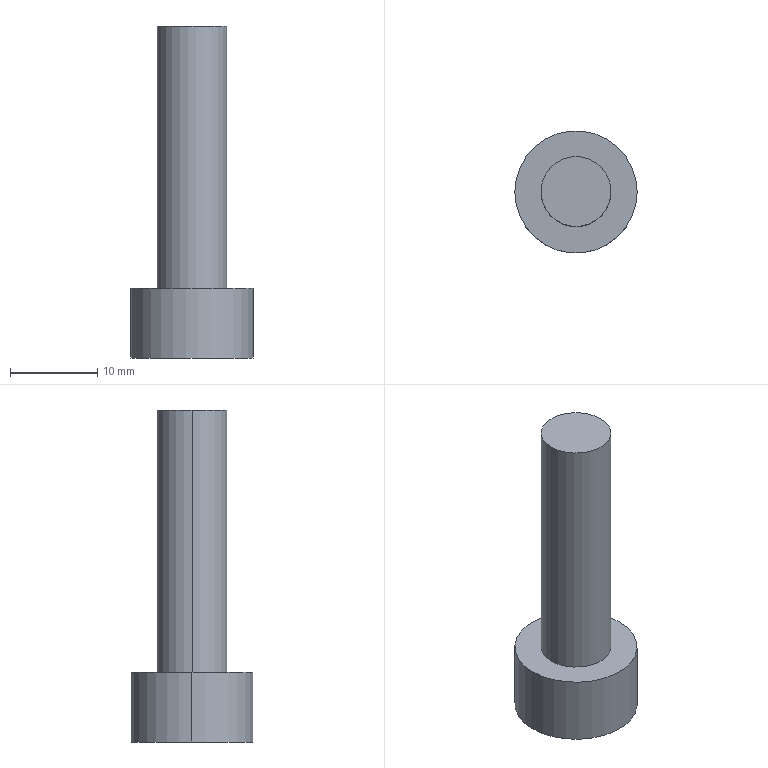Part | STEP file | LG M8_3F | 1 solid | 14 faces | box 14 x 14 x 38 mm | volume 2614 mm3 | plane 10 | cylinder 4 | commonest cylinder face diameters 8 x2 14 x2
STEP:
#1=CARTESIAN_POINT('',(0.,0.,0.));
#2=DIRECTION('',(0.,0.,1.));
#3=DIRECTION('',(1.,0.,0.));
#4=AXIS2_PLACEMENT_3D('',#1,#2,#3);
#5=CARTESIAN_POINT('',(4.,0.,30.));
#6=VERTEX_POINT('',#5);
#7=CARTESIAN_POINT('',(-4.,0.,30.));
#8=VERTEX_POINT('',#7);
#9=CARTESIAN_POINT('',(0.,0.,30.));
#10=DIRECTION('',(0.,0.,1.));
#11=DIRECTION('',(1.,0.,0.));
#12=AXIS2_PLACEMENT_3D('',#9,#10,#11);
#13=CIRCLE('',#12,4.);
#14=CARTESIAN_POINT('',(0.,0.,30.));
#15=DIRECTION('',(0.,0.,-1.));
#16=DIRECTION('',(-1.,0.,0.));
#17=AXIS2_PLACEMENT_3D('',#14,#15,#16);
#18=CYLINDRICAL_SURFACE('',#17,4.);
#19=CARTESIAN_POINT('',(3.142,0.));
#20=DIRECTION('',(-1.,0.));
#21=VECTOR('',#20,1.);
#22=LINE('',#19,#21);
#23=(GEOMETRIC_REPRESENTATION_CONTEXT(2)PARAMETRIC_REPRESENTATION_CONTEXT()REPRESENTATION_CONTEXT('',''));
#24=DEFINITIONAL_REPRESENTATION('',(#22),#23);
#25=PCURVE('',#18,#24);
#26=CARTESIAN_POINT('',(0.,0.,30.));
#27=DIRECTION('',(0.,0.,1.));
#28=DIRECTION('',(1.,0.,0.));
#29=AXIS2_PLACEMENT_3D('',#26,#27,#28);
#30=PLANE('',#29);
#31=CARTESIAN_POINT('',(0.,0.));
#32=DIRECTION('',(1.,0.));
#33=AXIS2_PLACEMENT_2D('',#31,#32);
#34=CIRCLE('',#33,4.);
#35=(GEOMETRIC_REPRESENTATION_CONTEXT(2)PARAMETRIC_REPRESENTATION_CONTEXT()REPRESENTATION_CONTEXT('',''));
#36=DEFINITIONAL_REPRESENTATION('',(#34),#35);
#37=PCURVE('',#30,#36);
#38=SURFACE_CURVE('',#13,(#25,#37),.PCURVE_S1.);
#39=EDGE_CURVE('',#6,#8,#38,.T.);
#40=ORIENTED_EDGE('',*,*,#39,.F.);
#41=CARTESIAN_POINT('',(4.,0.,0.));
#42=VERTEX_POINT('',#41);
#43=CARTESIAN_POINT('',(4.,0.,30.));
#44=DIRECTION('',(0.,0.,-1.));
#45=VECTOR('',#44,1.);
#46=LINE('',#43,#45);
#47=CARTESIAN_POINT('',(3.142,0.));
#48=DIRECTION('',(0.,1.));
#49=VECTOR('',#48,1.);
#50=LINE('',#47,#49);
#51=(GEOMETRIC_REPRESENTATION_CONTEXT(2)PARAMETRIC_REPRESENTATION_CONTEXT()REPRESENTATION_CONTEXT('',''));
#52=DEFINITIONAL_REPRESENTATION('',(#50),#51);
#53=PCURVE('',#18,#52);
#54=CARTESIAN_POINT('',(0.,0.,30.));
#55=DIRECTION('',(0.,0.,-1.));
#56=DIRECTION('',(-1.,0.,0.));
#57=AXIS2_PLACEMENT_3D('',#54,#55,#56);
#58=CYLINDRICAL_SURFACE('',#57,4.);
#59=CARTESIAN_POINT('',(3.142,0.));
#60=DIRECTION('',(0.,1.));
#61=VECTOR('',#60,1.);
#62=LINE('',#59,#61);
#63=(GEOMETRIC_REPRESENTATION_CONTEXT(2)PARAMETRIC_REPRESENTATION_CONTEXT()REPRESENTATION_CONTEXT('',''));
#64=DEFINITIONAL_REPRESENTATION('',(#62),#63);
#65=PCURVE('',#58,#64);
#66=SURFACE_CURVE('',#46,(#53,#65),.PCURVE_S1.);
#67=EDGE_CURVE('',#6,#42,#66,.T.);
#68=ORIENTED_EDGE('',*,*,#67,.T.);
#69=CARTESIAN_POINT('',(-4.,0.,0.));
#70=VERTEX_POINT('',#69);
#71=CARTESIAN_POINT('',(0.,0.,0.));
#72=DIRECTION('',(0.,0.,1.));
#73=DIRECTION('',(1.,0.,0.));
#74=AXIS2_PLACEMENT_3D('',#71,#72,#73);
#75=CIRCLE('',#74,4.);
#76=CARTESIAN_POINT('',(3.142,30.));
#77=DIRECTION('',(-1.,0.));
#78=VECTOR('',#77,1.);
#79=LINE('',#76,#78);
#80=(GEOMETRIC_REPRESENTATION_CONTEXT(2)PARAMETRIC_REPRESENTATION_CONTEXT()REPRESENTATION_CONTEXT('',''));
#81=DEFINITIONAL_REPRESENTATION('',(#79),#80);
#82=PCURVE('',#18,#81);
#83=CARTESIAN_POINT('',(0.,0.,0.));
#84=DIRECTION('',(0.,0.,1.));
#85=DIRECTION('',(1.,0.,0.));
#86=AXIS2_PLACEMENT_3D('',#83,#84,#85);
#87=PLANE('',#86);
#88=CARTESIAN_POINT('',(0.,0.));
#89=DIRECTION('',(1.,0.));
#90=AXIS2_PLACEMENT_2D('',#88,#89);
#91=CIRCLE('',#90,4.);
#92=(GEOMETRIC_REPRESENTATION_CONTEXT(2)PARAMETRIC_REPRESENTATION_CONTEXT()REPRESENTATION_CONTEXT('',''));
#93=DEFINITIONAL_REPRESENTATION('',(#91),#92);
#94=PCURVE('',#87,#93);
#95=SURFACE_CURVE('',#75,(#82,#94),.PCURVE_S1.);
#96=EDGE_CURVE('',#42,#70,#95,.T.);
#97=ORIENTED_EDGE('',*,*,#96,.T.);
#98=CARTESIAN_POINT('',(-4.,0.,30.));
#99=DIRECTION('',(0.,0.,-1.));
#100=VECTOR('',#99,1.);
#101=LINE('',#98,#100);
#102=CARTESIAN_POINT('',(0.,0.));
#103=DIRECTION('',(0.,1.));
#104=VECTOR('',#103,1.);
#105=LINE('',#102,#104);
#106=(GEOMETRIC_REPRESENTATION_CONTEXT(2)PARAMETRIC_REPRESENTATION_CONTEXT()REPRESENTATION_CONTEXT('',''));
#107=DEFINITIONAL_REPRESENTATION('',(#105),#106);
#108=PCURVE('',#18,#107);
#109=CARTESIAN_POINT('',(6.283,0.));
#110=DIRECTION('',(0.,1.));
#111=VECTOR('',#110,1.);
#112=LINE('',#109,#111);
#113=(GEOMETRIC_REPRESENTATION_CONTEXT(2)PARAMETRIC_REPRESENTATION_CONTEXT()REPRESENTATION_CONTEXT('',''));
#114=DEFINITIONAL_REPRESENTATION('',(#112),#113);
#115=PCURVE('',#58,#114);
#116=SURFACE_CURVE('',#101,(#108,#115),.PCURVE_S1.);
#117=EDGE_CURVE('',#8,#70,#116,.T.);
#118=ORIENTED_EDGE('',*,*,#117,.F.);
#119=EDGE_LOOP('',(#40,#68,#97,#118));
#120=FACE_BOUND('',#119,.T.);
#121=ADVANCED_FACE('',(#120),#18,.T.);
#122=CARTESIAN_POINT('',(7.,0.,-8.));
#123=VERTEX_POINT('',#122);
#124=CARTESIAN_POINT('',(-7.,0.,-8.));
#125=VERTEX_POINT('',#124);
#126=CARTESIAN_POINT('',(0.,0.,-8.));
#127=DIRECTION('',(0.,0.,1.));
#128=DIRECTION('',(1.,0.,0.));
#129=AXIS2_PLACEMENT_3D('',#126,#127,#128);
#130=CIRCLE('',#129,7.);
#131=CARTESIAN_POINT('',(0.,0.,-8.));
#132=DIRECTION('',(0.,0.,1.));
#133=DIRECTION('',(1.,0.,0.));
#134=AXIS2_PLACEMENT_3D('',#131,#132,#133);
#135=CYLINDRICAL_SURFACE('',#134,7.);
#136=CARTESIAN_POINT('',(0.,0.));
#137=DIRECTION('',(1.,0.));
#138=VECTOR('',#137,1.);
#139=LINE('',#136,#138);
#140=(GEOMETRIC_REPRESENTATION_CONTEXT(2)PARAMETRIC_REPRESENTATION_CONTEXT()REPRESENTATION_CONTEXT('',''));
#141=DEFINITIONAL_REPRESENTATION('',(#139),#140);
#142=PCURVE('',#135,#141);
#143=CARTESIAN_POINT('',(0.,0.,-8.));
#144=DIRECTION('',(0.,0.,1.));
#145=DIRECTION('',(1.,0.,0.));
#146=AXIS2_PLACEMENT_3D('',#143,#144,#145);
#147=PLANE('',#146);
#148=CARTESIAN_POINT('',(0.,0.));
#149=DIRECTION('',(1.,0.));
#150=AXIS2_PLACEMENT_2D('',#148,#149);
#151=CIRCLE('',#150,7.);
#152=(GEOMETRIC_REPRESENTATION_CONTEXT(2)PARAMETRIC_REPRESENTATION_CONTEXT()REPRESENTATION_CONTEXT('',''));
#153=DEFINITIONAL_REPRESENTATION('',(#151),#152);
#154=PCURVE('',#147,#153);
#155=SURFACE_CURVE('',#130,(#142,#154),.PCURVE_S1.);
#156=EDGE_CURVE('',#123,#125,#155,.T.);
#157=ORIENTED_EDGE('',*,*,#156,.T.);
#158=CARTESIAN_POINT('',(-7.,0.,0.));
#159=VERTEX_POINT('',#158);
#160=CARTESIAN_POINT('',(-7.,0.,-8.));
#161=DIRECTION('',(0.,0.,1.));
#162=VECTOR('',#161,1.);
#163=LINE('',#160,#162);
#164=CARTESIAN_POINT('',(3.142,0.));
#165=DIRECTION('',(0.,1.));
#166=VECTOR('',#165,1.);
#167=LINE('',#164,#166);
#168=(GEOMETRIC_REPRESENTATION_CONTEXT(2)PARAMETRIC_REPRESENTATION_CONTEXT()REPRESENTATION_CONTEXT('',''));
#169=DEFINITIONAL_REPRESENTATION('',(#167),#168);
#170=PCURVE('',#135,#169);
#171=CARTESIAN_POINT('',(0.,0.,-8.));
#172=DIRECTION('',(0.,0.,1.));
#173=DIRECTION('',(1.,0.,0.));
#174=AXIS2_PLACEMENT_3D('',#171,#172,#173);
#175=CYLINDRICAL_SURFACE('',#174,7.);
#176=CARTESIAN_POINT('',(3.142,0.));
#177=DIRECTION('',(0.,1.));
#178=VECTOR('',#177,1.);
#179=LINE('',#176,#178);
#180=(GEOMETRIC_REPRESENTATION_CONTEXT(2)PARAMETRIC_REPRESENTATION_CONTEXT()REPRESENTATION_CONTEXT('',''));
#181=DEFINITIONAL_REPRESENTATION('',(#179),#180);
#182=PCURVE('',#175,#181);
#183=SURFACE_CURVE('',#163,(#170,#182),.PCURVE_S1.);
#184=EDGE_CURVE('',#125,#159,#183,.T.);
#185=ORIENTED_EDGE('',*,*,#184,.T.);
#186=CARTESIAN_POINT('',(7.,0.,0.));
#187=VERTEX_POINT('',#186);
#188=CARTESIAN_POINT('',(0.,0.,0.));
#189=DIRECTION('',(0.,0.,1.));
#190=DIRECTION('',(1.,0.,0.));
#191=AXIS2_PLACEMENT_3D('',#188,#189,#190);
#192=CIRCLE('',#191,7.);
#193=CARTESIAN_POINT('',(0.,8.));
#194=DIRECTION('',(1.,0.));
#195=VECTOR('',#194,1.);
#196=LINE('',#193,#195);
#197=(GEOMETRIC_REPRESENTATION_CONTEXT(2)PARAMETRIC_REPRESENTATION_CONTEXT()REPRESENTATION_CONTEXT('',''));
#198=DEFINITIONAL_REPRESENTATION('',(#196),#197);
#199=PCURVE('',#135,#198);
#200=CARTESIAN_POINT('',(0.,0.));
#201=DIRECTION('',(1.,0.));
#202=AXIS2_PLACEMENT_2D('',#200,#201);
#203=CIRCLE('',#202,7.);
#204=(GEOMETRIC_REPRESENTATION_CONTEXT(2)PARAMETRIC_REPRESENTATION_CONTEXT()REPRESENTATION_CONTEXT('',''));
#205=DEFINITIONAL_REPRESENTATION('',(#203),#204);
#206=PCURVE('',#87,#205);
#207=SURFACE_CURVE('',#192,(#199,#206),.PCURVE_S1.);
#208=EDGE_CURVE('',#187,#159,#207,.T.);
#209=ORIENTED_EDGE('',*,*,#208,.F.);
#210=CARTESIAN_POINT('',(7.,0.,-8.));
#211=DIRECTION('',(0.,0.,1.));
#212=VECTOR('',#211,1.);
#213=LINE('',#210,#212);
#214=CARTESIAN_POINT('',(0.,0.));
#215=DIRECTION('',(0.,1.));
#216=VECTOR('',#215,1.);
#217=LINE('',#214,#216);
#218=(GEOMETRIC_REPRESENTATION_CONTEXT(2)PARAMETRIC_REPRESENTATION_CONTEXT()REPRESENTATION_CONTEXT('',''));
#219=DEFINITIONAL_REPRESENTATION('',(#217),#218);
#220=PCURVE('',#135,#219);
#221=CARTESIAN_POINT('',(6.283,0.));
#222=DIRECTION('',(0.,1.));
#223=VECTOR('',#222,1.);
#224=LINE('',#221,#223);
#225=(GEOMETRIC_REPRESENTATION_CONTEXT(2)PARAMETRIC_REPRESENTATION_CONTEXT()REPRESENTATION_CONTEXT('',''));
#226=DEFINITIONAL_REPRESENTATION('',(#224),#225);
#227=PCURVE('',#175,#226);
#228=SURFACE_CURVE('',#213,(#220,#227),.PCURVE_S1.);
#229=EDGE_CURVE('',#123,#187,#228,.T.);
#230=ORIENTED_EDGE('',*,*,#229,.F.);
#231=EDGE_LOOP('',(#157,#185,#209,#230));
#232=FACE_BOUND('',#231,.T.);
#233=ADVANCED_FACE('',(#232),#135,.T.);
#234=ORIENTED_EDGE('',*,*,#208,.T.);
#235=CARTESIAN_POINT('',(0.,0.,0.));
#236=DIRECTION('',(0.,0.,1.));
#237=DIRECTION('',(1.,0.,0.));
#238=AXIS2_PLACEMENT_3D('',#235,#236,#237);
#239=CIRCLE('',#238,7.);
#240=CARTESIAN_POINT('',(0.,0.));
#241=DIRECTION('',(1.,0.));
#242=AXIS2_PLACEMENT_2D('',#240,#241);
#243=CIRCLE('',#242,7.);
#244=(GEOMETRIC_REPRESENTATION_CONTEXT(2)PARAMETRIC_REPRESENTATION_CONTEXT()REPRESENTATION_CONTEXT('',''));
#245=DEFINITIONAL_REPRESENTATION('',(#243),#244);
#246=PCURVE('',#87,#245);
#247=CARTESIAN_POINT('',(0.,8.));
#248=DIRECTION('',(1.,0.));
#249=VECTOR('',#248,1.);
#250=LINE('',#247,#249);
#251=(GEOMETRIC_REPRESENTATION_CONTEXT(2)PARAMETRIC_REPRESENTATION_CONTEXT()REPRESENTATION_CONTEXT('',''));
#252=DEFINITIONAL_REPRESENTATION('',(#250),#251);
#253=PCURVE('',#175,#252);
#254=SURFACE_CURVE('',#239,(#246,#253),.PCURVE_S1.);
#255=EDGE_CURVE('',#159,#187,#254,.T.);
#256=ORIENTED_EDGE('',*,*,#255,.T.);
#257=EDGE_LOOP('',(#234,#256));
#258=FACE_BOUND('',#257,.T.);
#259=CARTESIAN_POINT('',(0.,0.,0.));
#260=DIRECTION('',(0.,0.,1.));
#261=DIRECTION('',(1.,0.,0.));
#262=AXIS2_PLACEMENT_3D('',#259,#260,#261);
#263=CIRCLE('',#262,4.);
#264=CARTESIAN_POINT('',(0.,0.));
#265=DIRECTION('',(1.,0.));
#266=AXIS2_PLACEMENT_2D('',#264,#265);
#267=CIRCLE('',#266,4.);
#268=(GEOMETRIC_REPRESENTATION_CONTEXT(2)PARAMETRIC_REPRESENTATION_CONTEXT()REPRESENTATION_CONTEXT('',''));
#269=DEFINITIONAL_REPRESENTATION('',(#267),#268);
#270=PCURVE('',#87,#269);
#271=CARTESIAN_POINT('',(9.425,30.));
#272=DIRECTION('',(-1.,0.));
#273=VECTOR('',#272,1.);
#274=LINE('',#271,#273);
#275=(GEOMETRIC_REPRESENTATION_CONTEXT(2)PARAMETRIC_REPRESENTATION_CONTEXT()REPRESENTATION_CONTEXT('',''));
#276=DEFINITIONAL_REPRESENTATION('',(#274),#275);
#277=PCURVE('',#58,#276);
#278=SURFACE_CURVE('',#263,(#270,#277),.PCURVE_S1.);
#279=EDGE_CURVE('',#70,#42,#278,.T.);
#280=ORIENTED_EDGE('',*,*,#279,.F.);
#281=ORIENTED_EDGE('',*,*,#96,.F.);
#282=EDGE_LOOP('',(#280,#281));
#283=FACE_BOUND('',#282,.T.);
#284=ADVANCED_FACE('',(#258,#283),#87,.T.);
#285=ORIENTED_EDGE('',*,*,#184,.F.);
#286=CARTESIAN_POINT('',(0.,0.,-8.));
#287=DIRECTION('',(0.,0.,1.));
#288=DIRECTION('',(1.,0.,0.));
#289=AXIS2_PLACEMENT_3D('',#286,#287,#288);
#290=CIRCLE('',#289,7.);
#291=CARTESIAN_POINT('',(0.,0.));
#292=DIRECTION('',(1.,0.));
#293=VECTOR('',#292,1.);
#294=LINE('',#291,#293);
#295=(GEOMETRIC_REPRESENTATION_CONTEXT(2)PARAMETRIC_REPRESENTATION_CONTEXT()REPRESENTATION_CONTEXT('',''));
#296=DEFINITIONAL_REPRESENTATION('',(#294),#295);
#297=PCURVE('',#175,#296);
#298=CARTESIAN_POINT('',(0.,0.));
#299=DIRECTION('',(1.,0.));
#300=AXIS2_PLACEMENT_2D('',#298,#299);
#301=CIRCLE('',#300,7.);
#302=(GEOMETRIC_REPRESENTATION_CONTEXT(2)PARAMETRIC_REPRESENTATION_CONTEXT()REPRESENTATION_CONTEXT('',''));
#303=DEFINITIONAL_REPRESENTATION('',(#301),#302);
#304=PCURVE('',#147,#303);
#305=SURFACE_CURVE('',#290,(#297,#304),.PCURVE_S1.);
#306=EDGE_CURVE('',#125,#123,#305,.T.);
#307=ORIENTED_EDGE('',*,*,#306,.T.);
#308=ORIENTED_EDGE('',*,*,#229,.T.);
#309=ORIENTED_EDGE('',*,*,#255,.F.);
#310=EDGE_LOOP('',(#285,#307,#308,#309));
#311=FACE_BOUND('',#310,.T.);
#312=ADVANCED_FACE('',(#311),#175,.T.);
#313=CARTESIAN_POINT('',(-3.476,0.,-8.));
#314=VERTEX_POINT('',#313);
#315=CARTESIAN_POINT('',(-1.738,3.01,-8.));
#316=VERTEX_POINT('',#315);
#317=CARTESIAN_POINT('',(-3.476,0.,-8.));
#318=DIRECTION('',(0.5,0.866,0.));
#319=VECTOR('',#318,1.);
#320=LINE('',#317,#319);
#321=CARTESIAN_POINT('',(-3.476,0.));
#322=DIRECTION('',(0.5,0.866));
#323=VECTOR('',#322,1.);
#324=LINE('',#321,#323);
#325=(GEOMETRIC_REPRESENTATION_CONTEXT(2)PARAMETRIC_REPRESENTATION_CONTEXT()REPRESENTATION_CONTEXT('',''));
#326=DEFINITIONAL_REPRESENTATION('',(#324),#325);
#327=PCURVE('',#147,#326);
#328=CARTESIAN_POINT('',(-3.476,0.,-4.));
#329=DIRECTION('',(-0.866,0.5,0.));
#330=DIRECTION('',(-0.5,-0.866,0.));
#331=AXIS2_PLACEMENT_3D('',#328,#329,#330);
#332=PLANE('',#331);
#333=CARTESIAN_POINT('',(0.,-4.));
#334=DIRECTION('',(-1.,0.));
#335=VECTOR('',#334,1.);
#336=LINE('',#333,#335);
#337=(GEOMETRIC_REPRESENTATION_CONTEXT(2)PARAMETRIC_REPRESENTATION_CONTEXT()REPRESENTATION_CONTEXT('',''));
#338=DEFINITIONAL_REPRESENTATION('',(#336),#337);
#339=PCURVE('',#332,#338);
#340=SURFACE_CURVE('',#320,(#327,#339),.PCURVE_S1.);
#341=EDGE_CURVE('',#314,#316,#340,.T.);
#342=ORIENTED_EDGE('',*,*,#341,.F.);
#343=CARTESIAN_POINT('',(-1.738,-3.01,-8.));
#344=VERTEX_POINT('',#343);
#345=CARTESIAN_POINT('',(-1.738,-3.01,-8.));
#346=DIRECTION('',(-0.5,0.866,0.));
#347=VECTOR('',#346,1.);
#348=LINE('',#345,#347);
#349=CARTESIAN_POINT('',(-1.738,-3.01));
#350=DIRECTION('',(-0.5,0.866));
#351=VECTOR('',#350,1.);
#352=LINE('',#349,#351);
#353=(GEOMETRIC_REPRESENTATION_CONTEXT(2)PARAMETRIC_REPRESENTATION_CONTEXT()REPRESENTATION_CONTEXT('',''));
#354=DEFINITIONAL_REPRESENTATION('',(#352),#353);
#355=PCURVE('',#147,#354);
#356=CARTESIAN_POINT('',(-1.738,-3.01,-4.));
#357=DIRECTION('',(-0.866,-0.5,0.));
#358=DIRECTION('',(0.5,-0.866,0.));
#359=AXIS2_PLACEMENT_3D('',#356,#357,#358);
#360=PLANE('',#359);
#361=CARTESIAN_POINT('',(0.,-4.));
#362=DIRECTION('',(-1.,0.));
#363=VECTOR('',#362,1.);
#364=LINE('',#361,#363);
#365=(GEOMETRIC_REPRESENTATION_CONTEXT(2)PARAMETRIC_REPRESENTATION_CONTEXT()REPRESENTATION_CONTEXT('',''));
#366=DEFINITIONAL_REPRESENTATION('',(#364),#365);
#367=PCURVE('',#360,#366);
#368=SURFACE_CURVE('',#348,(#355,#367),.PCURVE_S1.);
#369=EDGE_CURVE('',#344,#314,#368,.T.);
#370=ORIENTED_EDGE('',*,*,#369,.F.);
#371=CARTESIAN_POINT('',(1.738,-3.01,-8.));
#372=VERTEX_POINT('',#371);
#373=CARTESIAN_POINT('',(1.738,-3.01,-8.));
#374=DIRECTION('',(-1.,0.,0.));
#375=VECTOR('',#374,1.);
#376=LINE('',#373,#375);
#377=CARTESIAN_POINT('',(1.738,-3.01));
#378=DIRECTION('',(-1.,0.));
#379=VECTOR('',#378,1.);
#380=LINE('',#377,#379);
#381=(GEOMETRIC_REPRESENTATION_CONTEXT(2)PARAMETRIC_REPRESENTATION_CONTEXT()REPRESENTATION_CONTEXT('',''));
#382=DEFINITIONAL_REPRESENTATION('',(#380),#381);
#383=PCURVE('',#147,#382);
#384=CARTESIAN_POINT('',(1.738,-3.01,-4.));
#385=DIRECTION('',(0.,-1.,0.));
#386=DIRECTION('',(0.,0.,-1.));
#387=AXIS2_PLACEMENT_3D('',#384,#385,#386);
#388=PLANE('',#387);
#389=CARTESIAN_POINT('',(4.,0.));
#390=DIRECTION('',(0.,-1.));
#391=VECTOR('',#390,1.);
#392=LINE('',#389,#391);
#393=(GEOMETRIC_REPRESENTATION_CONTEXT(2)PARAMETRIC_REPRESENTATION_CONTEXT()REPRESENTATION_CONTEXT('',''));
#394=DEFINITIONAL_REPRESENTATION('',(#392),#393);
#395=PCURVE('',#388,#394);
#396=SURFACE_CURVE('',#376,(#383,#395),.PCURVE_S1.);
#397=EDGE_CURVE('',#372,#344,#396,.T.);
#398=ORIENTED_EDGE('',*,*,#397,.F.);
#399=CARTESIAN_POINT('',(3.476,0.,-8.));
#400=VERTEX_POINT('',#399);
#401=CARTESIAN_POINT('',(3.476,0.,-8.));
#402=DIRECTION('',(-0.5,-0.866,0.));
#403=VECTOR('',#402,1.);
#404=LINE('',#401,#403);
#405=CARTESIAN_POINT('',(3.476,0.));
#406=DIRECTION('',(-0.5,-0.866));
#407=VECTOR('',#406,1.);
#408=LINE('',#405,#407);
#409=(GEOMETRIC_REPRESENTATION_CONTEXT(2)PARAMETRIC_REPRESENTATION_CONTEXT()REPRESENTATION_CONTEXT('',''));
#410=DEFINITIONAL_REPRESENTATION('',(#408),#409);
#411=PCURVE('',#147,#410);
#412=CARTESIAN_POINT('',(3.476,0.,-4.));
#413=DIRECTION('',(0.866,-0.5,0.));
#414=DIRECTION('',(0.5,0.866,0.));
#415=AXIS2_PLACEMENT_3D('',#412,#413,#414);
#416=PLANE('',#415);
#417=CARTESIAN_POINT('',(0.,-4.));
#418=DIRECTION('',(-1.,0.));
#419=VECTOR('',#418,1.);
#420=LINE('',#417,#419);
#421=(GEOMETRIC_REPRESENTATION_CONTEXT(2)PARAMETRIC_REPRESENTATION_CONTEXT()REPRESENTATION_CONTEXT('',''));
#422=DEFINITIONAL_REPRESENTATION('',(#420),#421);
#423=PCURVE('',#416,#422);
#424=SURFACE_CURVE('',#404,(#411,#423),.PCURVE_S1.);
#425=EDGE_CURVE('',#400,#372,#424,.T.);
#426=ORIENTED_EDGE('',*,*,#425,.F.);
#427=CARTESIAN_POINT('',(1.738,3.01,-8.));
#428=VERTEX_POINT('',#427);
#429=CARTESIAN_POINT('',(1.738,3.01,-8.));
#430=DIRECTION('',(0.5,-0.866,0.));
#431=VECTOR('',#430,1.);
#432=LINE('',#429,#431);
#433=CARTESIAN_POINT('',(1.738,3.01));
#434=DIRECTION('',(0.5,-0.866));
#435=VECTOR('',#434,1.);
#436=LINE('',#433,#435);
#437=(GEOMETRIC_REPRESENTATION_CONTEXT(2)PARAMETRIC_REPRESENTATION_CONTEXT()REPRESENTATION_CONTEXT('',''));
#438=DEFINITIONAL_REPRESENTATION('',(#436),#437);
#439=PCURVE('',#147,#438);
#440=CARTESIAN_POINT('',(1.738,3.01,-4.));
#441=DIRECTION('',(0.866,0.5,0.));
#442=DIRECTION('',(-0.5,0.866,0.));
#443=AXIS2_PLACEMENT_3D('',#440,#441,#442);
#444=PLANE('',#443);
#445=CARTESIAN_POINT('',(0.,-4.));
#446=DIRECTION('',(-1.,0.));
#447=VECTOR('',#446,1.);
#448=LINE('',#445,#447);
#449=(GEOMETRIC_REPRESENTATION_CONTEXT(2)PARAMETRIC_REPRESENTATION_CONTEXT()REPRESENTATION_CONTEXT('',''));
#450=DEFINITIONAL_REPRESENTATION('',(#448),#449);
#451=PCURVE('',#444,#450);
#452=SURFACE_CURVE('',#432,(#439,#451),.PCURVE_S1.);
#453=EDGE_CURVE('',#428,#400,#452,.T.);
#454=ORIENTED_EDGE('',*,*,#453,.F.);
#455=CARTESIAN_POINT('',(-1.738,3.01,-8.));
#456=DIRECTION('',(1.,0.,0.));
#457=VECTOR('',#456,1.);
#458=LINE('',#455,#457);
#459=CARTESIAN_POINT('',(-1.738,3.01));
#460=DIRECTION('',(1.,0.));
#461=VECTOR('',#460,1.);
#462=LINE('',#459,#461);
#463=(GEOMETRIC_REPRESENTATION_CONTEXT(2)PARAMETRIC_REPRESENTATION_CONTEXT()REPRESENTATION_CONTEXT('',''));
#464=DEFINITIONAL_REPRESENTATION('',(#462),#463);
#465=PCURVE('',#147,#464);
#466=CARTESIAN_POINT('',(-1.738,3.01,-4.));
#467=DIRECTION('',(0.,1.,0.));
#468=DIRECTION('',(0.,0.,1.));
#469=AXIS2_PLACEMENT_3D('',#466,#467,#468);
#470=PLANE('',#469);
#471=CARTESIAN_POINT('',(-4.,0.));
#472=DIRECTION('',(0.,1.));
#473=VECTOR('',#472,1.);
#474=LINE('',#471,#473);
#475=(GEOMETRIC_REPRESENTATION_CONTEXT(2)PARAMETRIC_REPRESENTATION_CONTEXT()REPRESENTATION_CONTEXT('',''));
#476=DEFINITIONAL_REPRESENTATION('',(#474),#475);
#477=PCURVE('',#470,#476);
#478=SURFACE_CURVE('',#458,(#465,#477),.PCURVE_S1.);
#479=EDGE_CURVE('',#316,#428,#478,.T.);
#480=ORIENTED_EDGE('',*,*,#479,.F.);
#481=EDGE_LOOP('',(#342,#370,#398,#426,#454,#480));
#482=FACE_BOUND('',#481,.T.);
#483=ORIENTED_EDGE('',*,*,#156,.F.);
#484=ORIENTED_EDGE('',*,*,#306,.F.);
#485=EDGE_LOOP('',(#483,#484));
#486=FACE_BOUND('',#485,.T.);
#487=ADVANCED_FACE('',(#482,#486),#147,.F.);
#488=ORIENTED_EDGE('',*,*,#67,.F.);
#489=CARTESIAN_POINT('',(0.,0.,30.));
#490=DIRECTION('',(0.,0.,1.));
#491=DIRECTION('',(1.,0.,0.));
#492=AXIS2_PLACEMENT_3D('',#489,#490,#491);
#493=CIRCLE('',#492,4.);
#494=CARTESIAN_POINT('',(9.425,0.));
#495=DIRECTION('',(-1.,0.));
#496=VECTOR('',#495,1.);
#497=LINE('',#494,#496);
#498=(GEOMETRIC_REPRESENTATION_CONTEXT(2)PARAMETRIC_REPRESENTATION_CONTEXT()REPRESENTATION_CONTEXT('',''));
#499=DEFINITIONAL_REPRESENTATION('',(#497),#498);
#500=PCURVE('',#58,#499);
#501=CARTESIAN_POINT('',(0.,0.));
#502=DIRECTION('',(1.,0.));
#503=AXIS2_PLACEMENT_2D('',#501,#502);
#504=CIRCLE('',#503,4.);
#505=(GEOMETRIC_REPRESENTATION_CONTEXT(2)PARAMETRIC_REPRESENTATION_CONTEXT()REPRESENTATION_CONTEXT('',''));
#506=DEFINITIONAL_REPRESENTATION('',(#504),#505);
#507=PCURVE('',#30,#506);
#508=SURFACE_CURVE('',#493,(#500,#507),.PCURVE_S1.);
#509=EDGE_CURVE('',#8,#6,#508,.T.);
#510=ORIENTED_EDGE('',*,*,#509,.F.);
#511=ORIENTED_EDGE('',*,*,#117,.T.);
#512=ORIENTED_EDGE('',*,*,#279,.T.);
#513=EDGE_LOOP('',(#488,#510,#511,#512));
#514=FACE_BOUND('',#513,.T.);
#515=ADVANCED_FACE('',(#514),#58,.T.);
#516=ORIENTED_EDGE('',*,*,#509,.T.);
#517=ORIENTED_EDGE('',*,*,#39,.T.);
#518=EDGE_LOOP('',(#516,#517));
#519=FACE_BOUND('',#518,.T.);
#520=ADVANCED_FACE('',(#519),#30,.T.);
#521=ORIENTED_EDGE('',*,*,#369,.T.);
#522=CARTESIAN_POINT('',(-3.476,0.,-4.));
#523=VERTEX_POINT('',#522);
#524=CARTESIAN_POINT('',(-3.476,0.,-4.));
#525=DIRECTION('',(0.,0.,-1.));
#526=VECTOR('',#525,1.);
#527=LINE('',#524,#526);
#528=CARTESIAN_POINT('',(-3.476,0.));
#529=DIRECTION('',(0.,-1.));
#530=VECTOR('',#529,1.);
#531=LINE('',#528,#530);
#532=(GEOMETRIC_REPRESENTATION_CONTEXT(2)PARAMETRIC_REPRESENTATION_CONTEXT()REPRESENTATION_CONTEXT('',''));
#533=DEFINITIONAL_REPRESENTATION('',(#531),#532);
#534=PCURVE('',#360,#533);
#535=CARTESIAN_POINT('',(0.,0.));
#536=DIRECTION('',(0.,-1.));
#537=VECTOR('',#536,1.);
#538=LINE('',#535,#537);
#539=(GEOMETRIC_REPRESENTATION_CONTEXT(2)PARAMETRIC_REPRESENTATION_CONTEXT()REPRESENTATION_CONTEXT('',''));
#540=DEFINITIONAL_REPRESENTATION('',(#538),#539);
#541=PCURVE('',#332,#540);
#542=SURFACE_CURVE('',#527,(#534,#541),.PCURVE_S1.);
#543=EDGE_CURVE('',#523,#314,#542,.T.);
#544=ORIENTED_EDGE('',*,*,#543,.F.);
#545=CARTESIAN_POINT('',(-1.738,-3.01,-4.));
#546=VERTEX_POINT('',#545);
#547=CARTESIAN_POINT('',(-1.738,-3.01,-4.));
#548=DIRECTION('',(-0.5,0.866,0.));
#549=VECTOR('',#548,1.);
#550=LINE('',#547,#549);
#551=CARTESIAN_POINT('',(0.,0.));
#552=DIRECTION('',(-1.,0.));
#553=VECTOR('',#552,1.);
#554=LINE('',#551,#553);
#555=(GEOMETRIC_REPRESENTATION_CONTEXT(2)PARAMETRIC_REPRESENTATION_CONTEXT()REPRESENTATION_CONTEXT('',''));
#556=DEFINITIONAL_REPRESENTATION('',(#554),#555);
#557=PCURVE('',#360,#556);
#558=CARTESIAN_POINT('',(0.,0.,-4.));
#559=DIRECTION('',(0.,0.,-1.));
#560=DIRECTION('',(-1.,0.,0.));
#561=AXIS2_PLACEMENT_3D('',#558,#559,#560);
#562=PLANE('',#561);
#563=CARTESIAN_POINT('',(1.738,-3.01));
#564=DIRECTION('',(0.5,0.866));
#565=VECTOR('',#564,1.);
#566=LINE('',#563,#565);
#567=(GEOMETRIC_REPRESENTATION_CONTEXT(2)PARAMETRIC_REPRESENTATION_CONTEXT()REPRESENTATION_CONTEXT('',''));
#568=DEFINITIONAL_REPRESENTATION('',(#566),#567);
#569=PCURVE('',#562,#568);
#570=SURFACE_CURVE('',#550,(#557,#569),.PCURVE_S1.);
#571=EDGE_CURVE('',#546,#523,#570,.T.);
#572=ORIENTED_EDGE('',*,*,#571,.F.);
#573=CARTESIAN_POINT('',(-1.738,-3.01,-4.));
#574=DIRECTION('',(0.,0.,-1.));
#575=VECTOR('',#574,1.);
#576=LINE('',#573,#575);
#577=CARTESIAN_POINT('',(0.,0.));
#578=DIRECTION('',(0.,-1.));
#579=VECTOR('',#578,1.);
#580=LINE('',#577,#579);
#581=(GEOMETRIC_REPRESENTATION_CONTEXT(2)PARAMETRIC_REPRESENTATION_CONTEXT()REPRESENTATION_CONTEXT('',''));
#582=DEFINITIONAL_REPRESENTATION('',(#580),#581);
#583=PCURVE('',#360,#582);
#584=CARTESIAN_POINT('',(0.,-3.476));
#585=DIRECTION('',(1.,0.));
#586=VECTOR('',#585,1.);
#587=LINE('',#584,#586);
#588=(GEOMETRIC_REPRESENTATION_CONTEXT(2)PARAMETRIC_REPRESENTATION_CONTEXT()REPRESENTATION_CONTEXT('',''));
#589=DEFINITIONAL_REPRESENTATION('',(#587),#588);
#590=PCURVE('',#388,#589);
#591=SURFACE_CURVE('',#576,(#583,#590),.PCURVE_S1.);
#592=EDGE_CURVE('',#546,#344,#591,.T.);
#593=ORIENTED_EDGE('',*,*,#592,.T.);
#594=EDGE_LOOP('',(#521,#544,#572,#593));
#595=FACE_BOUND('',#594,.T.);
#596=ADVANCED_FACE('',(#595),#360,.F.);
#597=ORIENTED_EDGE('',*,*,#397,.T.);
#598=ORIENTED_EDGE('',*,*,#592,.F.);
#599=CARTESIAN_POINT('',(1.738,-3.01,-4.));
#600=VERTEX_POINT('',#599);
#601=CARTESIAN_POINT('',(1.738,-3.01,-4.));
#602=DIRECTION('',(-1.,0.,0.));
#603=VECTOR('',#602,1.);
#604=LINE('',#601,#603);
#605=CARTESIAN_POINT('',(0.,0.));
#606=DIRECTION('',(0.,-1.));
#607=VECTOR('',#606,1.);
#608=LINE('',#605,#607);
#609=(GEOMETRIC_REPRESENTATION_CONTEXT(2)PARAMETRIC_REPRESENTATION_CONTEXT()REPRESENTATION_CONTEXT('',''));
#610=DEFINITIONAL_REPRESENTATION('',(#608),#609);
#611=PCURVE('',#388,#610);
#612=CARTESIAN_POINT('',(-1.738,-3.01));
#613=DIRECTION('',(1.,0.));
#614=VECTOR('',#613,1.);
#615=LINE('',#612,#614);
#616=(GEOMETRIC_REPRESENTATION_CONTEXT(2)PARAMETRIC_REPRESENTATION_CONTEXT()REPRESENTATION_CONTEXT('',''));
#617=DEFINITIONAL_REPRESENTATION('',(#615),#616);
#618=PCURVE('',#562,#617);
#619=SURFACE_CURVE('',#604,(#611,#618),.PCURVE_S1.);
#620=EDGE_CURVE('',#600,#546,#619,.T.);
#621=ORIENTED_EDGE('',*,*,#620,.F.);
#622=CARTESIAN_POINT('',(1.738,-3.01,-4.));
#623=DIRECTION('',(0.,0.,-1.));
#624=VECTOR('',#623,1.);
#625=LINE('',#622,#624);
#626=CARTESIAN_POINT('',(0.,0.));
#627=DIRECTION('',(1.,0.));
#628=VECTOR('',#627,1.);
#629=LINE('',#626,#628);
#630=(GEOMETRIC_REPRESENTATION_CONTEXT(2)PARAMETRIC_REPRESENTATION_CONTEXT()REPRESENTATION_CONTEXT('',''));
#631=DEFINITIONAL_REPRESENTATION('',(#629),#630);
#632=PCURVE('',#388,#631);
#633=CARTESIAN_POINT('',(-3.476,0.));
#634=DIRECTION('',(0.,-1.));
#635=VECTOR('',#634,1.);
#636=LINE('',#633,#635);
#637=(GEOMETRIC_REPRESENTATION_CONTEXT(2)PARAMETRIC_REPRESENTATION_CONTEXT()REPRESENTATION_CONTEXT('',''));
#638=DEFINITIONAL_REPRESENTATION('',(#636),#637);
#639=PCURVE('',#416,#638);
#640=SURFACE_CURVE('',#625,(#632,#639),.PCURVE_S1.);
#641=EDGE_CURVE('',#600,#372,#640,.T.);
#642=ORIENTED_EDGE('',*,*,#641,.T.);
#643=EDGE_LOOP('',(#597,#598,#621,#642));
#644=FACE_BOUND('',#643,.T.);
#645=ADVANCED_FACE('',(#644),#388,.F.);
#646=ORIENTED_EDGE('',*,*,#425,.T.);
#647=ORIENTED_EDGE('',*,*,#641,.F.);
#648=CARTESIAN_POINT('',(3.476,0.,-4.));
#649=VERTEX_POINT('',#648);
#650=CARTESIAN_POINT('',(3.476,0.,-4.));
#651=DIRECTION('',(-0.5,-0.866,0.));
#652=VECTOR('',#651,1.);
#653=LINE('',#650,#652);
#654=CARTESIAN_POINT('',(0.,0.));
#655=DIRECTION('',(-1.,0.));
#656=VECTOR('',#655,1.);
#657=LINE('',#654,#656);
#658=(GEOMETRIC_REPRESENTATION_CONTEXT(2)PARAMETRIC_REPRESENTATION_CONTEXT()REPRESENTATION_CONTEXT('',''));
#659=DEFINITIONAL_REPRESENTATION('',(#657),#658);
#660=PCURVE('',#416,#659);
#661=CARTESIAN_POINT('',(-3.476,0.));
#662=DIRECTION('',(0.5,-0.866));
#663=VECTOR('',#662,1.);
#664=LINE('',#661,#663);
#665=(GEOMETRIC_REPRESENTATION_CONTEXT(2)PARAMETRIC_REPRESENTATION_CONTEXT()REPRESENTATION_CONTEXT('',''));
#666=DEFINITIONAL_REPRESENTATION('',(#664),#665);
#667=PCURVE('',#562,#666);
#668=SURFACE_CURVE('',#653,(#660,#667),.PCURVE_S1.);
#669=EDGE_CURVE('',#649,#600,#668,.T.);
#670=ORIENTED_EDGE('',*,*,#669,.F.);
#671=CARTESIAN_POINT('',(3.476,0.,-4.));
#672=DIRECTION('',(0.,0.,-1.));
#673=VECTOR('',#672,1.);
#674=LINE('',#671,#673);
#675=CARTESIAN_POINT('',(0.,0.));
#676=DIRECTION('',(0.,-1.));
#677=VECTOR('',#676,1.);
#678=LINE('',#675,#677);
#679=(GEOMETRIC_REPRESENTATION_CONTEXT(2)PARAMETRIC_REPRESENTATION_CONTEXT()REPRESENTATION_CONTEXT('',''));
#680=DEFINITIONAL_REPRESENTATION('',(#678),#679);
#681=PCURVE('',#416,#680);
#682=CARTESIAN_POINT('',(-3.476,0.));
#683=DIRECTION('',(0.,-1.));
#684=VECTOR('',#683,1.);
#685=LINE('',#682,#684);
#686=(GEOMETRIC_REPRESENTATION_CONTEXT(2)PARAMETRIC_REPRESENTATION_CONTEXT()REPRESENTATION_CONTEXT('',''));
#687=DEFINITIONAL_REPRESENTATION('',(#685),#686);
#688=PCURVE('',#444,#687);
#689=SURFACE_CURVE('',#674,(#681,#688),.PCURVE_S1.);
#690=EDGE_CURVE('',#649,#400,#689,.T.);
#691=ORIENTED_EDGE('',*,*,#690,.T.);
#692=EDGE_LOOP('',(#646,#647,#670,#691));
#693=FACE_BOUND('',#692,.T.);
#694=ADVANCED_FACE('',(#693),#416,.F.);
#695=ORIENTED_EDGE('',*,*,#453,.T.);
#696=ORIENTED_EDGE('',*,*,#690,.F.);
#697=CARTESIAN_POINT('',(1.738,3.01,-4.));
#698=VERTEX_POINT('',#697);
#699=CARTESIAN_POINT('',(1.738,3.01,-4.));
#700=DIRECTION('',(0.5,-0.866,0.));
#701=VECTOR('',#700,1.);
#702=LINE('',#699,#701);
#703=CARTESIAN_POINT('',(0.,0.));
#704=DIRECTION('',(-1.,0.));
#705=VECTOR('',#704,1.);
#706=LINE('',#703,#705);
#707=(GEOMETRIC_REPRESENTATION_CONTEXT(2)PARAMETRIC_REPRESENTATION_CONTEXT()REPRESENTATION_CONTEXT('',''));
#708=DEFINITIONAL_REPRESENTATION('',(#706),#707);
#709=PCURVE('',#444,#708);
#710=CARTESIAN_POINT('',(-1.738,3.01));
#711=DIRECTION('',(-0.5,-0.866));
#712=VECTOR('',#711,1.);
#713=LINE('',#710,#712);
#714=(GEOMETRIC_REPRESENTATION_CONTEXT(2)PARAMETRIC_REPRESENTATION_CONTEXT()REPRESENTATION_CONTEXT('',''));
#715=DEFINITIONAL_REPRESENTATION('',(#713),#714);
#716=PCURVE('',#562,#715);
#717=SURFACE_CURVE('',#702,(#709,#716),.PCURVE_S1.);
#718=EDGE_CURVE('',#698,#649,#717,.T.);
#719=ORIENTED_EDGE('',*,*,#718,.F.);
#720=CARTESIAN_POINT('',(1.738,3.01,-4.));
#721=DIRECTION('',(0.,0.,-1.));
#722=VECTOR('',#721,1.);
#723=LINE('',#720,#722);
#724=CARTESIAN_POINT('',(0.,0.));
#725=DIRECTION('',(0.,-1.));
#726=VECTOR('',#725,1.);
#727=LINE('',#724,#726);
#728=(GEOMETRIC_REPRESENTATION_CONTEXT(2)PARAMETRIC_REPRESENTATION_CONTEXT()REPRESENTATION_CONTEXT('',''));
#729=DEFINITIONAL_REPRESENTATION('',(#727),#728);
#730=PCURVE('',#444,#729);
#731=CARTESIAN_POINT('',(0.,3.476));
#732=DIRECTION('',(-1.,0.));
#733=VECTOR('',#732,1.);
#734=LINE('',#731,#733);
#735=(GEOMETRIC_REPRESENTATION_CONTEXT(2)PARAMETRIC_REPRESENTATION_CONTEXT()REPRESENTATION_CONTEXT('',''));
#736=DEFINITIONAL_REPRESENTATION('',(#734),#735);
#737=PCURVE('',#470,#736);
#738=SURFACE_CURVE('',#723,(#730,#737),.PCURVE_S1.);
#739=EDGE_CURVE('',#698,#428,#738,.T.);
#740=ORIENTED_EDGE('',*,*,#739,.T.);
#741=EDGE_LOOP('',(#695,#696,#719,#740));
#742=FACE_BOUND('',#741,.T.);
#743=ADVANCED_FACE('',(#742),#444,.F.);
#744=ORIENTED_EDGE('',*,*,#479,.T.);
#745=ORIENTED_EDGE('',*,*,#739,.F.);
#746=CARTESIAN_POINT('',(-1.738,3.01,-4.));
#747=VERTEX_POINT('',#746);
#748=CARTESIAN_POINT('',(-1.738,3.01,-4.));
#749=DIRECTION('',(1.,0.,0.));
#750=VECTOR('',#749,1.);
#751=LINE('',#748,#750);
#752=CARTESIAN_POINT('',(0.,0.));
#753=DIRECTION('',(0.,1.));
#754=VECTOR('',#753,1.);
#755=LINE('',#752,#754);
#756=(GEOMETRIC_REPRESENTATION_CONTEXT(2)PARAMETRIC_REPRESENTATION_CONTEXT()REPRESENTATION_CONTEXT('',''));
#757=DEFINITIONAL_REPRESENTATION('',(#755),#756);
#758=PCURVE('',#470,#757);
#759=CARTESIAN_POINT('',(1.738,3.01));
#760=DIRECTION('',(-1.,0.));
#761=VECTOR('',#760,1.);
#762=LINE('',#759,#761);
#763=(GEOMETRIC_REPRESENTATION_CONTEXT(2)PARAMETRIC_REPRESENTATION_CONTEXT()REPRESENTATION_CONTEXT('',''));
#764=DEFINITIONAL_REPRESENTATION('',(#762),#763);
#765=PCURVE('',#562,#764);
#766=SURFACE_CURVE('',#751,(#758,#765),.PCURVE_S1.);
#767=EDGE_CURVE('',#747,#698,#766,.T.);
#768=ORIENTED_EDGE('',*,*,#767,.F.);
#769=CARTESIAN_POINT('',(-1.738,3.01,-4.));
#770=DIRECTION('',(0.,0.,-1.));
#771=VECTOR('',#770,1.);
#772=LINE('',#769,#771);
#773=CARTESIAN_POINT('',(0.,0.));
#774=DIRECTION('',(-1.,0.));
#775=VECTOR('',#774,1.);
#776=LINE('',#773,#775);
#777=(GEOMETRIC_REPRESENTATION_CONTEXT(2)PARAMETRIC_REPRESENTATION_CONTEXT()REPRESENTATION_CONTEXT('',''));
#778=DEFINITIONAL_REPRESENTATION('',(#776),#777);
#779=PCURVE('',#470,#778);
#780=CARTESIAN_POINT('',(-3.476,0.));
#781=DIRECTION('',(0.,-1.));
#782=VECTOR('',#781,1.);
#783=LINE('',#780,#782);
#784=(GEOMETRIC_REPRESENTATION_CONTEXT(2)PARAMETRIC_REPRESENTATION_CONTEXT()REPRESENTATION_CONTEXT('',''));
#785=DEFINITIONAL_REPRESENTATION('',(#783),#784);
#786=PCURVE('',#332,#785);
#787=SURFACE_CURVE('',#772,(#779,#786),.PCURVE_S1.);
#788=EDGE_CURVE('',#747,#316,#787,.T.);
#789=ORIENTED_EDGE('',*,*,#788,.T.);
#790=EDGE_LOOP('',(#744,#745,#768,#789));
#791=FACE_BOUND('',#790,.T.);
#792=ADVANCED_FACE('',(#791),#470,.F.);
#793=ORIENTED_EDGE('',*,*,#341,.T.);
#794=ORIENTED_EDGE('',*,*,#788,.F.);
#795=CARTESIAN_POINT('',(-3.476,0.,-4.));
#796=DIRECTION('',(0.5,0.866,0.));
#797=VECTOR('',#796,1.);
#798=LINE('',#795,#797);
#799=CARTESIAN_POINT('',(0.,0.));
#800=DIRECTION('',(-1.,0.));
#801=VECTOR('',#800,1.);
#802=LINE('',#799,#801);
#803=(GEOMETRIC_REPRESENTATION_CONTEXT(2)PARAMETRIC_REPRESENTATION_CONTEXT()REPRESENTATION_CONTEXT('',''));
#804=DEFINITIONAL_REPRESENTATION('',(#802),#803);
#805=PCURVE('',#332,#804);
#806=CARTESIAN_POINT('',(3.476,0.));
#807=DIRECTION('',(-0.5,0.866));
#808=VECTOR('',#807,1.);
#809=LINE('',#806,#808);
#810=(GEOMETRIC_REPRESENTATION_CONTEXT(2)PARAMETRIC_REPRESENTATION_CONTEXT()REPRESENTATION_CONTEXT('',''));
#811=DEFINITIONAL_REPRESENTATION('',(#809),#810);
#812=PCURVE('',#562,#811);
#813=SURFACE_CURVE('',#798,(#805,#812),.PCURVE_S1.);
#814=EDGE_CURVE('',#523,#747,#813,.T.);
#815=ORIENTED_EDGE('',*,*,#814,.F.);
#816=ORIENTED_EDGE('',*,*,#543,.T.);
#817=EDGE_LOOP('',(#793,#794,#815,#816));
#818=FACE_BOUND('',#817,.T.);
#819=ADVANCED_FACE('',(#818),#332,.F.);
#820=ORIENTED_EDGE('',*,*,#571,.T.);
#821=ORIENTED_EDGE('',*,*,#814,.T.);
#822=ORIENTED_EDGE('',*,*,#767,.T.);
#823=ORIENTED_EDGE('',*,*,#718,.T.);
#824=ORIENTED_EDGE('',*,*,#669,.T.);
#825=ORIENTED_EDGE('',*,*,#620,.T.);
#826=EDGE_LOOP('',(#820,#821,#822,#823,#824,#825));
#827=FACE_BOUND('',#826,.T.);
#828=ADVANCED_FACE('',(#827),#562,.T.);
#829=CLOSED_SHELL('',(#121,#233,#284,#312,#487,#515,#520,#596,#645,#694,#743,#792,#819,#828));
#830=MANIFOLD_SOLID_BREP('',#829);
#831=(LENGTH_UNIT()NAMED_UNIT(*)SI_UNIT(.MILLI.,.METRE.));
#832=UNCERTAINTY_MEASURE_WITH_UNIT(LENGTH_MEASURE(0.0000001),#831,'','');
#833=(NAMED_UNIT(*)PLANE_ANGLE_UNIT()SI_UNIT($,.RADIAN.));
#834=(NAMED_UNIT(*)SI_UNIT($,.STERADIAN.)SOLID_ANGLE_UNIT());
#835=(GEOMETRIC_REPRESENTATION_CONTEXT(3)GLOBAL_UNCERTAINTY_ASSIGNED_CONTEXT((#832))GLOBAL_UNIT_ASSIGNED_CONTEXT((#831,#833,#834))REPRESENTATION_CONTEXT('',''));
#836=ADVANCED_BREP_SHAPE_REPRESENTATION('',(#4,#830),#835);